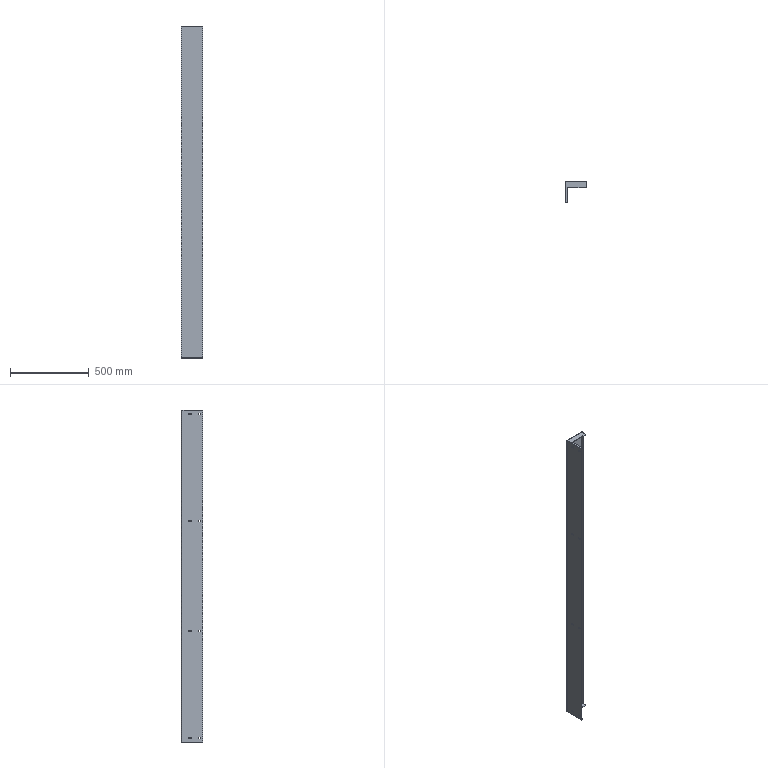Part | SolidWorks | features FlatPattern 3, SMBaseFlange 3, SheetMetal 3, ICE 1 | 3 solids | 78 faces | box 135 x 135 x 2110 mm | volume 1800450 mm3 | plane 58 | cylinder 20 | commonest cylinder face diameters 8 x16 1.473 x2 7.473 x2